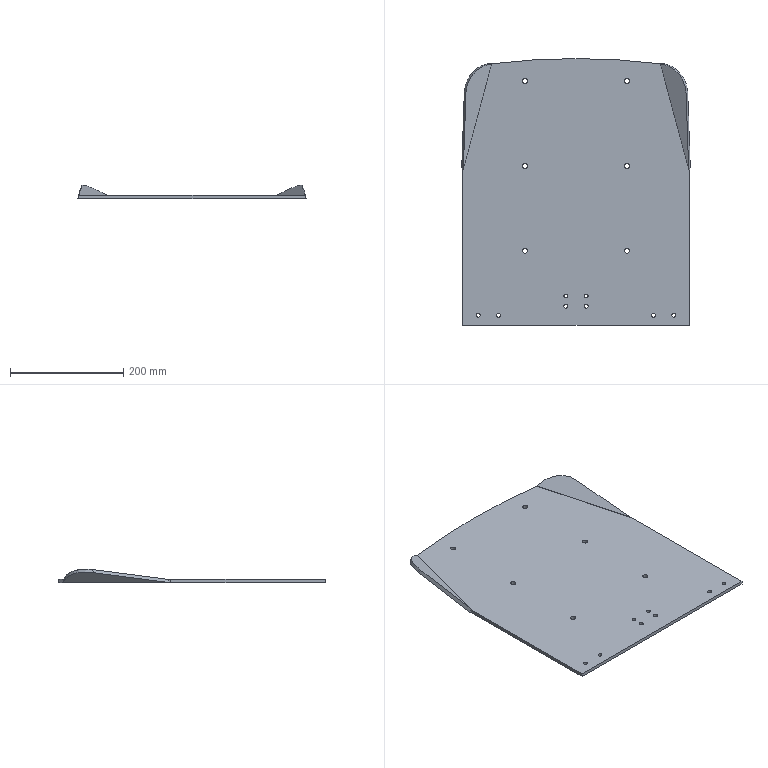Part | SolidWorks | features HoleWzd 3, Fillet 2, ICE 2, SM3dBend 2, FlatPattern 1, SMBaseFlange 1, SheetMetal 1 | 1 solid | 53 faces | box 403.952 x 471.784 x 24.242 mm | volume 1111640 mm3 | cylinder 38 | plane 11 | spline 4 | commonest cylinder face diameters 7 x16 9 x12 100 x3 2400 x3 1 x2 13 x2